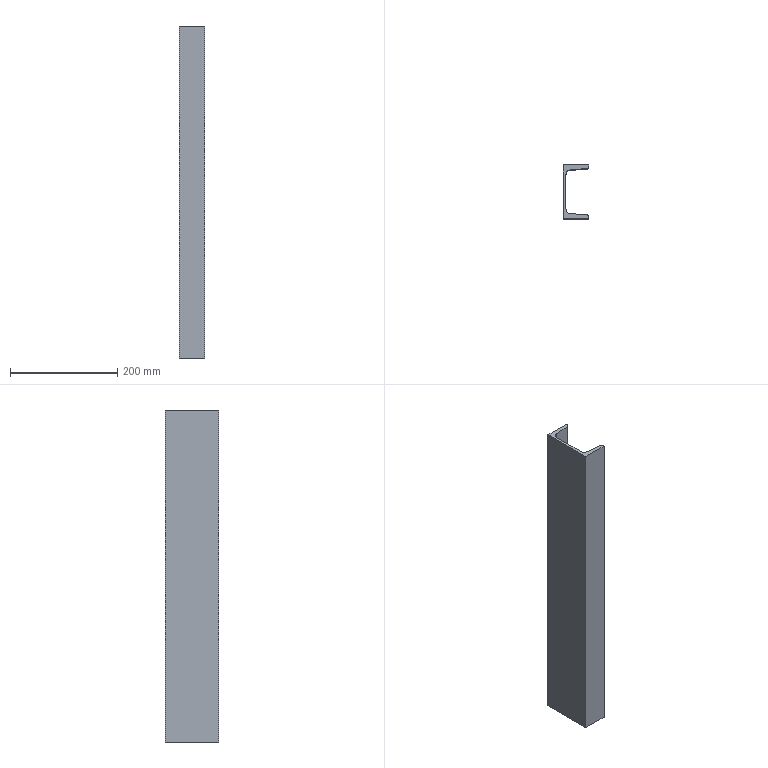Part | NX | features BREP 1 | 1 solid | 20 faces | box 48 x 100 x 620 mm | volume 770701 mm3 | cylinder 10 | plane 10 | commonest cylinder face diameters 14 x6 8.4 x2 17 x2
STEP:
#1=CARTESIAN_POINT('',(30.,92.079,-177.));
#2=VERTEX_POINT('',#1);
#3=CARTESIAN_POINT('',(30.,92.079,-163.));
#4=VERTEX_POINT('',#3);
#5=CARTESIAN_POINT('',(30.,92.079,-177.));
#6=CARTESIAN_POINT('',(16.,90.926,-177.));
#7=CARTESIAN_POINT('',(16.,90.926,-163.));
#8=CARTESIAN_POINT('',(30.,92.079,-163.));
#9=(BOUNDED_CURVE()B_SPLINE_CURVE(3,(#5,#6,#7,#8),.UNSPECIFIED.,.F.,.F.)B_SPLINE_CURVE_WITH_KNOTS((4,4),(0.,1.),.PIECEWISE_BEZIER_KNOTS.)CURVE()GEOMETRIC_REPRESENTATION_ITEM()RATIONAL_B_SPLINE_CURVE((1.,0.3333,0.3333,1.))REPRESENTATION_ITEM(''));
#10=EDGE_CURVE('',#2,#4,#9,.T.);
#11=ORIENTED_EDGE('',*,*,#10,.F.);
#12=CARTESIAN_POINT('',(30.,100.,-177.));
#13=VERTEX_POINT('',#12);
#14=CARTESIAN_POINT('',(30.,70.,-177.));
#15=DIRECTION('',(0.,1.,0.));
#16=VECTOR('',#15,1000.);
#17=LINE('',#14,#16);
#18=EDGE_CURVE('',#2,#13,#17,.T.);
#19=ORIENTED_EDGE('',*,*,#18,.T.);
#20=CARTESIAN_POINT('',(30.,100.,-163.));
#21=VERTEX_POINT('',#20);
#22=CARTESIAN_POINT('',(30.,100.,-170.));
#23=DIRECTION('',(0.,1.,0.));
#24=DIRECTION('',(0.,0.,1.));
#25=AXIS2_PLACEMENT_3D('',#22,#23,#24);
#26=CIRCLE('',#25,7.);
#27=EDGE_CURVE('',#13,#21,#26,.T.);
#28=ORIENTED_EDGE('',*,*,#27,.T.);
#29=CARTESIAN_POINT('',(30.,70.,-163.));
#30=DIRECTION('',(0.,1.,0.));
#31=VECTOR('',#30,1000.);
#32=LINE('',#29,#31);
#33=EDGE_CURVE('',#4,#21,#32,.T.);
#34=ORIENTED_EDGE('',*,*,#33,.F.);
#35=EDGE_LOOP('',(#11,#19,#28,#34));
#36=FACE_BOUND('',#35,.T.);
#37=CARTESIAN_POINT('',(30.,70.,-170.));
#38=DIRECTION('',(0.,1.,0.));
#39=DIRECTION('',(0.,0.,-1.));
#40=AXIS2_PLACEMENT_3D('',#37,#38,#39);
#41=CYLINDRICAL_SURFACE('',#40,7.);
#42=ADVANCED_FACE('',(#36),#41,.F.);
#43=CARTESIAN_POINT('',(30.,92.079,163.));
#44=VERTEX_POINT('',#43);
#45=CARTESIAN_POINT('',(30.,92.079,177.));
#46=VERTEX_POINT('',#45);
#47=CARTESIAN_POINT('',(30.,92.079,163.));
#48=CARTESIAN_POINT('',(16.,90.926,163.));
#49=CARTESIAN_POINT('',(16.,90.926,177.));
#50=CARTESIAN_POINT('',(30.,92.079,177.));
#51=(BOUNDED_CURVE()B_SPLINE_CURVE(3,(#47,#48,#49,#50),.UNSPECIFIED.,.F.,.F.)B_SPLINE_CURVE_WITH_KNOTS((4,4),(0.,1.),.PIECEWISE_BEZIER_KNOTS.)CURVE()GEOMETRIC_REPRESENTATION_ITEM()RATIONAL_B_SPLINE_CURVE((1.,0.3333,0.3333,1.))REPRESENTATION_ITEM(''));
#52=EDGE_CURVE('',#44,#46,#51,.T.);
#53=ORIENTED_EDGE('',*,*,#52,.F.);
#54=CARTESIAN_POINT('',(30.,100.,163.));
#55=VERTEX_POINT('',#54);
#56=CARTESIAN_POINT('',(30.,70.,163.));
#57=DIRECTION('',(0.,1.,0.));
#58=VECTOR('',#57,1000.);
#59=LINE('',#56,#58);
#60=EDGE_CURVE('',#44,#55,#59,.T.);
#61=ORIENTED_EDGE('',*,*,#60,.T.);
#62=CARTESIAN_POINT('',(30.,100.,177.));
#63=VERTEX_POINT('',#62);
#64=CARTESIAN_POINT('',(30.,100.,170.));
#65=DIRECTION('',(0.,1.,0.));
#66=DIRECTION('',(0.,0.,1.));
#67=AXIS2_PLACEMENT_3D('',#64,#65,#66);
#68=CIRCLE('',#67,7.);
#69=EDGE_CURVE('',#55,#63,#68,.T.);
#70=ORIENTED_EDGE('',*,*,#69,.T.);
#71=CARTESIAN_POINT('',(30.,70.,177.));
#72=DIRECTION('',(0.,1.,0.));
#73=VECTOR('',#72,1000.);
#74=LINE('',#71,#73);
#75=EDGE_CURVE('',#46,#63,#74,.T.);
#76=ORIENTED_EDGE('',*,*,#75,.F.);
#77=EDGE_LOOP('',(#53,#61,#70,#76));
#78=FACE_BOUND('',#77,.T.);
#79=CARTESIAN_POINT('',(30.,70.,170.));
#80=DIRECTION('',(0.,1.,0.));
#81=DIRECTION('',(0.,0.,-1.));
#82=AXIS2_PLACEMENT_3D('',#79,#80,#81);
#83=CYLINDRICAL_SURFACE('',#82,7.);
#84=ADVANCED_FACE('',(#78),#83,.F.);
#85=CARTESIAN_POINT('',(30.,92.079,-7.));
#86=VERTEX_POINT('',#85);
#87=CARTESIAN_POINT('',(30.,92.079,7.));
#88=VERTEX_POINT('',#87);
#89=CARTESIAN_POINT('',(30.,92.079,-7.));
#90=CARTESIAN_POINT('',(16.,90.926,-7.));
#91=CARTESIAN_POINT('',(16.,90.926,7.));
#92=CARTESIAN_POINT('',(30.,92.079,7.));
#93=(BOUNDED_CURVE()B_SPLINE_CURVE(3,(#89,#90,#91,#92),.UNSPECIFIED.,.F.,.F.)B_SPLINE_CURVE_WITH_KNOTS((4,4),(0.,1.),.PIECEWISE_BEZIER_KNOTS.)CURVE()GEOMETRIC_REPRESENTATION_ITEM()RATIONAL_B_SPLINE_CURVE((1.,0.3333,0.3333,1.))REPRESENTATION_ITEM(''));
#94=EDGE_CURVE('',#86,#88,#93,.T.);
#95=ORIENTED_EDGE('',*,*,#94,.F.);
#96=CARTESIAN_POINT('',(30.,100.,-7.));
#97=VERTEX_POINT('',#96);
#98=CARTESIAN_POINT('',(30.,70.,-7.));
#99=DIRECTION('',(0.,1.,0.));
#100=VECTOR('',#99,1000.);
#101=LINE('',#98,#100);
#102=EDGE_CURVE('',#86,#97,#101,.T.);
#103=ORIENTED_EDGE('',*,*,#102,.T.);
#104=CARTESIAN_POINT('',(30.,100.,7.));
#105=VERTEX_POINT('',#104);
#106=CARTESIAN_POINT('',(30.,100.,0.));
#107=DIRECTION('',(0.,1.,0.));
#108=DIRECTION('',(0.,0.,1.));
#109=AXIS2_PLACEMENT_3D('',#106,#107,#108);
#110=CIRCLE('',#109,7.);
#111=EDGE_CURVE('',#97,#105,#110,.T.);
#112=ORIENTED_EDGE('',*,*,#111,.T.);
#113=CARTESIAN_POINT('',(30.,70.,7.));
#114=DIRECTION('',(0.,1.,0.));
#115=VECTOR('',#114,1000.);
#116=LINE('',#113,#115);
#117=EDGE_CURVE('',#88,#105,#116,.T.);
#118=ORIENTED_EDGE('',*,*,#117,.F.);
#119=EDGE_LOOP('',(#95,#103,#112,#118));
#120=FACE_BOUND('',#119,.T.);
#121=CARTESIAN_POINT('',(30.,70.,0.));
#122=DIRECTION('',(0.,1.,0.));
#123=DIRECTION('',(0.,0.,-1.));
#124=AXIS2_PLACEMENT_3D('',#121,#122,#123);
#125=CYLINDRICAL_SURFACE('',#124,7.);
#126=ADVANCED_FACE('',(#120),#125,.F.);
#127=CARTESIAN_POINT('',(0.,0.,-310.));
#128=VERTEX_POINT('',#127);
#129=CARTESIAN_POINT('',(48.,0.,-310.));
#130=VERTEX_POINT('',#129);
#131=CARTESIAN_POINT('',(0.,0.,-310.));
#132=DIRECTION('',(1.,0.,0.));
#133=VECTOR('',#132,1000.);
#134=LINE('',#131,#133);
#135=EDGE_CURVE('',#128,#130,#134,.T.);
#136=ORIENTED_EDGE('',*,*,#135,.T.);
#137=CARTESIAN_POINT('',(48.,0.,310.));
#138=VERTEX_POINT('',#137);
#139=CARTESIAN_POINT('',(48.,0.,310.));
#140=DIRECTION('',(0.,0.,-1.));
#141=VECTOR('',#140,1000.);
#142=LINE('',#139,#141);
#143=EDGE_CURVE('',#138,#130,#142,.T.);
#144=ORIENTED_EDGE('',*,*,#143,.F.);
#145=CARTESIAN_POINT('',(0.,0.,310.));
#146=VERTEX_POINT('',#145);
#147=CARTESIAN_POINT('',(0.,0.,310.));
#148=DIRECTION('',(1.,0.,0.));
#149=VECTOR('',#148,1000.);
#150=LINE('',#147,#149);
#151=EDGE_CURVE('',#146,#138,#150,.T.);
#152=ORIENTED_EDGE('',*,*,#151,.F.);
#153=CARTESIAN_POINT('',(0.,0.,310.));
#154=DIRECTION('',(0.,0.,-1.));
#155=VECTOR('',#154,1000.);
#156=LINE('',#153,#155);
#157=EDGE_CURVE('',#146,#128,#156,.T.);
#158=ORIENTED_EDGE('',*,*,#157,.T.);
#159=EDGE_LOOP('',(#136,#144,#152,#158));
#160=FACE_BOUND('',#159,.T.);
#161=CARTESIAN_POINT('',(0.,0.,310.));
#162=DIRECTION('',(0.,1.,0.));
#163=DIRECTION('',(0.,0.,-1.));
#164=AXIS2_PLACEMENT_3D('',#161,#162,#163);
#165=PLANE('',#164);
#166=ADVANCED_FACE('',(#160),#165,.F.);
#167=CARTESIAN_POINT('',(48.,2.585,-310.));
#168=VERTEX_POINT('',#167);
#169=CARTESIAN_POINT('',(48.,0.,-310.));
#170=DIRECTION('',(0.,1.,0.));
#171=VECTOR('',#170,1000.);
#172=LINE('',#169,#171);
#173=EDGE_CURVE('',#130,#168,#172,.T.);
#174=ORIENTED_EDGE('',*,*,#173,.T.);
#175=CARTESIAN_POINT('',(48.,2.585,310.));
#176=VERTEX_POINT('',#175);
#177=CARTESIAN_POINT('',(48.,2.585,310.));
#178=DIRECTION('',(0.,0.,-1.));
#179=VECTOR('',#178,1000.);
#180=LINE('',#177,#179);
#181=EDGE_CURVE('',#176,#168,#180,.T.);
#182=ORIENTED_EDGE('',*,*,#181,.F.);
#183=CARTESIAN_POINT('',(48.,0.,310.));
#184=DIRECTION('',(0.,1.,0.));
#185=VECTOR('',#184,1000.);
#186=LINE('',#183,#185);
#187=EDGE_CURVE('',#138,#176,#186,.T.);
#188=ORIENTED_EDGE('',*,*,#187,.F.);
#189=ORIENTED_EDGE('',*,*,#143,.T.);
#190=EDGE_LOOP('',(#174,#182,#188,#189));
#191=FACE_BOUND('',#190,.T.);
#192=CARTESIAN_POINT('',(48.,0.,310.));
#193=DIRECTION('',(-1.,0.,0.));
#194=DIRECTION('',(0.,0.,-1.));
#195=AXIS2_PLACEMENT_3D('',#192,#193,#194);
#196=PLANE('',#195);
#197=ADVANCED_FACE('',(#191),#196,.F.);
#198=CARTESIAN_POINT('',(43.8,6.785,-310.));
#199=VERTEX_POINT('',#198);
#200=CARTESIAN_POINT('',(43.8,2.585,-310.));
#201=DIRECTION('',(0.,0.,1.));
#202=DIRECTION('',(1.,0.,0.));
#203=AXIS2_PLACEMENT_3D('',#200,#201,#202);
#204=CIRCLE('',#203,4.2);
#205=EDGE_CURVE('',#168,#199,#204,.T.);
#206=ORIENTED_EDGE('',*,*,#205,.T.);
#207=CARTESIAN_POINT('',(43.8,6.785,310.));
#208=VERTEX_POINT('',#207);
#209=CARTESIAN_POINT('',(43.8,6.785,310.));
#210=DIRECTION('',(0.,0.,-1.));
#211=VECTOR('',#210,1000.);
#212=LINE('',#209,#211);
#213=EDGE_CURVE('',#208,#199,#212,.T.);
#214=ORIENTED_EDGE('',*,*,#213,.F.);
#215=CARTESIAN_POINT('',(43.8,2.585,310.));
#216=DIRECTION('',(0.,0.,1.));
#217=DIRECTION('',(1.,0.,0.));
#218=AXIS2_PLACEMENT_3D('',#215,#216,#217);
#219=CIRCLE('',#218,4.2);
#220=EDGE_CURVE('',#176,#208,#219,.T.);
#221=ORIENTED_EDGE('',*,*,#220,.F.);
#222=ORIENTED_EDGE('',*,*,#181,.T.);
#223=EDGE_LOOP('',(#206,#214,#221,#222));
#224=FACE_BOUND('',#223,.T.);
#225=CARTESIAN_POINT('',(43.8,2.585,310.));
#226=DIRECTION('',(0.,0.,-1.));
#227=DIRECTION('',(1.,0.,0.));
#228=AXIS2_PLACEMENT_3D('',#225,#226,#227);
#229=CYLINDRICAL_SURFACE('',#228,4.2);
#230=ADVANCED_FACE('',(#224),#229,.T.);
#231=CARTESIAN_POINT('',(13.8,9.255,-310.));
#232=VERTEX_POINT('',#231);
#233=CARTESIAN_POINT('',(43.8,6.785,-310.));
#234=DIRECTION('',(-0.9966,0.08206,0.));
#235=VECTOR('',#234,1000.);
#236=LINE('',#233,#235);
#237=EDGE_CURVE('',#199,#232,#236,.T.);
#238=ORIENTED_EDGE('',*,*,#237,.T.);
#239=CARTESIAN_POINT('',(13.8,9.255,310.));
#240=VERTEX_POINT('',#239);
#241=CARTESIAN_POINT('',(13.8,9.255,310.));
#242=DIRECTION('',(0.,0.,-1.));
#243=VECTOR('',#242,1000.);
#244=LINE('',#241,#243);
#245=EDGE_CURVE('',#240,#232,#244,.T.);
#246=ORIENTED_EDGE('',*,*,#245,.F.);
#247=CARTESIAN_POINT('',(43.8,6.785,310.));
#248=DIRECTION('',(-0.9966,0.08206,0.));
#249=VECTOR('',#248,1000.);
#250=LINE('',#247,#249);
#251=EDGE_CURVE('',#208,#240,#250,.T.);
#252=ORIENTED_EDGE('',*,*,#251,.F.);
#253=ORIENTED_EDGE('',*,*,#213,.T.);
#254=EDGE_LOOP('',(#238,#246,#252,#253));
#255=FACE_BOUND('',#254,.T.);
#256=CARTESIAN_POINT('',(43.8,6.785,310.));
#257=DIRECTION('',(-0.08206,-0.9966,0.));
#258=DIRECTION('',(-0.9966,0.08206,0.));
#259=AXIS2_PLACEMENT_3D('',#256,#257,#258);
#260=PLANE('',#259);
#261=ADVANCED_FACE('',(#255),#260,.F.);
#262=CARTESIAN_POINT('',(5.3,17.755,-310.));
#263=VERTEX_POINT('',#262);
#264=CARTESIAN_POINT('',(13.8,17.755,-310.));
#265=DIRECTION('',(0.,0.,-1.));
#266=DIRECTION('',(1.,0.,0.));
#267=AXIS2_PLACEMENT_3D('',#264,#265,#266);
#268=CIRCLE('',#267,8.5);
#269=EDGE_CURVE('',#232,#263,#268,.T.);
#270=ORIENTED_EDGE('',*,*,#269,.T.);
#271=CARTESIAN_POINT('',(5.3,17.755,310.));
#272=VERTEX_POINT('',#271);
#273=CARTESIAN_POINT('',(5.3,17.755,310.));
#274=DIRECTION('',(0.,0.,-1.));
#275=VECTOR('',#274,1000.);
#276=LINE('',#273,#275);
#277=EDGE_CURVE('',#272,#263,#276,.T.);
#278=ORIENTED_EDGE('',*,*,#277,.F.);
#279=CARTESIAN_POINT('',(13.8,17.755,310.));
#280=DIRECTION('',(0.,0.,-1.));
#281=DIRECTION('',(1.,0.,0.));
#282=AXIS2_PLACEMENT_3D('',#279,#280,#281);
#283=CIRCLE('',#282,8.5);
#284=EDGE_CURVE('',#240,#272,#283,.T.);
#285=ORIENTED_EDGE('',*,*,#284,.F.);
#286=ORIENTED_EDGE('',*,*,#245,.T.);
#287=EDGE_LOOP('',(#270,#278,#285,#286));
#288=FACE_BOUND('',#287,.T.);
#289=CARTESIAN_POINT('',(13.8,17.755,310.));
#290=DIRECTION('',(0.,0.,-1.));
#291=DIRECTION('',(1.,0.,0.));
#292=AXIS2_PLACEMENT_3D('',#289,#290,#291);
#293=CYLINDRICAL_SURFACE('',#292,8.5);
#294=ADVANCED_FACE('',(#288),#293,.F.);
#295=CARTESIAN_POINT('',(5.3,82.245,-310.));
#296=VERTEX_POINT('',#295);
#297=CARTESIAN_POINT('',(5.3,17.755,-310.));
#298=DIRECTION('',(0.,1.,0.));
#299=VECTOR('',#298,1000.);
#300=LINE('',#297,#299);
#301=EDGE_CURVE('',#263,#296,#300,.T.);
#302=ORIENTED_EDGE('',*,*,#301,.T.);
#303=CARTESIAN_POINT('',(5.3,82.245,310.));
#304=VERTEX_POINT('',#303);
#305=CARTESIAN_POINT('',(5.3,82.245,310.));
#306=DIRECTION('',(0.,0.,-1.));
#307=VECTOR('',#306,1000.);
#308=LINE('',#305,#307);
#309=EDGE_CURVE('',#304,#296,#308,.T.);
#310=ORIENTED_EDGE('',*,*,#309,.F.);
#311=CARTESIAN_POINT('',(5.3,17.755,310.));
#312=DIRECTION('',(0.,1.,0.));
#313=VECTOR('',#312,1000.);
#314=LINE('',#311,#313);
#315=EDGE_CURVE('',#272,#304,#314,.T.);
#316=ORIENTED_EDGE('',*,*,#315,.F.);
#317=ORIENTED_EDGE('',*,*,#277,.T.);
#318=EDGE_LOOP('',(#302,#310,#316,#317));
#319=FACE_BOUND('',#318,.T.);
#320=CARTESIAN_POINT('',(5.3,17.755,310.));
#321=DIRECTION('',(-1.,0.,0.));
#322=DIRECTION('',(0.,0.,-1.));
#323=AXIS2_PLACEMENT_3D('',#320,#321,#322);
#324=PLANE('',#323);
#325=ADVANCED_FACE('',(#319),#324,.F.);
#326=CARTESIAN_POINT('',(13.8,90.745,-310.));
#327=VERTEX_POINT('',#326);
#328=CARTESIAN_POINT('',(13.8,82.245,-310.));
#329=DIRECTION('',(0.,0.,-1.));
#330=DIRECTION('',(-1.,0.,0.));
#331=AXIS2_PLACEMENT_3D('',#328,#329,#330);
#332=CIRCLE('',#331,8.5);
#333=EDGE_CURVE('',#296,#327,#332,.T.);
#334=ORIENTED_EDGE('',*,*,#333,.T.);
#335=CARTESIAN_POINT('',(13.8,90.745,310.));
#336=VERTEX_POINT('',#335);
#337=CARTESIAN_POINT('',(13.8,90.745,310.));
#338=DIRECTION('',(0.,0.,-1.));
#339=VECTOR('',#338,1000.);
#340=LINE('',#337,#339);
#341=EDGE_CURVE('',#336,#327,#340,.T.);
#342=ORIENTED_EDGE('',*,*,#341,.F.);
#343=CARTESIAN_POINT('',(13.8,82.245,310.));
#344=DIRECTION('',(0.,0.,-1.));
#345=DIRECTION('',(-1.,0.,0.));
#346=AXIS2_PLACEMENT_3D('',#343,#344,#345);
#347=CIRCLE('',#346,8.5);
#348=EDGE_CURVE('',#304,#336,#347,.T.);
#349=ORIENTED_EDGE('',*,*,#348,.F.);
#350=ORIENTED_EDGE('',*,*,#309,.T.);
#351=EDGE_LOOP('',(#334,#342,#349,#350));
#352=FACE_BOUND('',#351,.T.);
#353=CARTESIAN_POINT('',(13.8,82.245,310.));
#354=DIRECTION('',(0.,0.,-1.));
#355=DIRECTION('',(1.,0.,0.));
#356=AXIS2_PLACEMENT_3D('',#353,#354,#355);
#357=CYLINDRICAL_SURFACE('',#356,8.5);
#358=ADVANCED_FACE('',(#352),#357,.F.);
#359=CARTESIAN_POINT('',(30.,92.079,-163.));
#360=CARTESIAN_POINT('',(44.,93.231,-163.));
#361=CARTESIAN_POINT('',(44.,93.231,-177.));
#362=CARTESIAN_POINT('',(30.,92.079,-177.));
#363=(BOUNDED_CURVE()B_SPLINE_CURVE(3,(#359,#360,#361,#362),.UNSPECIFIED.,.F.,.F.)B_SPLINE_CURVE_WITH_KNOTS((4,4),(0.,1.),.PIECEWISE_BEZIER_KNOTS.)CURVE()GEOMETRIC_REPRESENTATION_ITEM()RATIONAL_B_SPLINE_CURVE((1.,0.3333,0.3333,1.))REPRESENTATION_ITEM(''));
#364=EDGE_CURVE('',#4,#2,#363,.T.);
#365=ORIENTED_EDGE('',*,*,#364,.T.);
#366=ORIENTED_EDGE('',*,*,#10,.T.);
#367=EDGE_LOOP('',(#365,#366));
#368=FACE_BOUND('',#367,.T.);
#369=CARTESIAN_POINT('',(30.,92.079,177.));
#370=CARTESIAN_POINT('',(44.,93.231,177.));
#371=CARTESIAN_POINT('',(44.,93.231,163.));
#372=CARTESIAN_POINT('',(30.,92.079,163.));
#373=(BOUNDED_CURVE()B_SPLINE_CURVE(3,(#369,#370,#371,#372),.UNSPECIFIED.,.F.,.F.)B_SPLINE_CURVE_WITH_KNOTS((4,4),(0.,1.),.PIECEWISE_BEZIER_KNOTS.)CURVE()GEOMETRIC_REPRESENTATION_ITEM()RATIONAL_B_SPLINE_CURVE((1.,0.3333,0.3333,1.))REPRESENTATION_ITEM(''));
#374=EDGE_CURVE('',#46,#44,#373,.T.);
#375=ORIENTED_EDGE('',*,*,#374,.T.);
#376=ORIENTED_EDGE('',*,*,#52,.T.);
#377=EDGE_LOOP('',(#375,#376));
#378=FACE_BOUND('',#377,.T.);
#379=CARTESIAN_POINT('',(30.,92.079,7.));
#380=CARTESIAN_POINT('',(44.,93.231,7.));
#381=CARTESIAN_POINT('',(44.,93.231,-7.));
#382=CARTESIAN_POINT('',(30.,92.079,-7.));
#383=(BOUNDED_CURVE()B_SPLINE_CURVE(3,(#379,#380,#381,#382),.UNSPECIFIED.,.F.,.F.)B_SPLINE_CURVE_WITH_KNOTS((4,4),(0.,1.),.PIECEWISE_BEZIER_KNOTS.)CURVE()GEOMETRIC_REPRESENTATION_ITEM()RATIONAL_B_SPLINE_CURVE((1.,0.3333,0.3333,1.))REPRESENTATION_ITEM(''));
#384=EDGE_CURVE('',#88,#86,#383,.T.);
#385=ORIENTED_EDGE('',*,*,#384,.T.);
#386=ORIENTED_EDGE('',*,*,#94,.T.);
#387=EDGE_LOOP('',(#385,#386));
#388=FACE_BOUND('',#387,.T.);
#389=CARTESIAN_POINT('',(43.8,93.215,-310.));
#390=VERTEX_POINT('',#389);
#391=CARTESIAN_POINT('',(43.8,93.215,-310.));
#392=DIRECTION('',(0.9966,0.08206,0.));
#393=VECTOR('',#392,1000.);
#394=LINE('',#391,#393);
#395=EDGE_CURVE('',#327,#390,#394,.T.);
#396=ORIENTED_EDGE('',*,*,#395,.T.);
#397=CARTESIAN_POINT('',(43.8,93.215,310.));
#398=VERTEX_POINT('',#397);
#399=CARTESIAN_POINT('',(43.8,93.215,310.));
#400=DIRECTION('',(0.,0.,-1.));
#401=VECTOR('',#400,1000.);
#402=LINE('',#399,#401);
#403=EDGE_CURVE('',#398,#390,#402,.T.);
#404=ORIENTED_EDGE('',*,*,#403,.F.);
#405=CARTESIAN_POINT('',(43.8,93.215,310.));
#406=DIRECTION('',(0.9966,0.08206,0.));
#407=VECTOR('',#406,1000.);
#408=LINE('',#405,#407);
#409=EDGE_CURVE('',#336,#398,#408,.T.);
#410=ORIENTED_EDGE('',*,*,#409,.F.);
#411=ORIENTED_EDGE('',*,*,#341,.T.);
#412=EDGE_LOOP('',(#396,#404,#410,#411));
#413=FACE_BOUND('',#412,.T.);
#414=CARTESIAN_POINT('',(43.8,93.215,310.));
#415=DIRECTION('',(-0.08206,0.9966,0.));
#416=DIRECTION('',(0.9966,0.08206,0.));
#417=AXIS2_PLACEMENT_3D('',#414,#415,#416);
#418=PLANE('',#417);
#419=ADVANCED_FACE('',(#368,#378,#388,#413),#418,.F.);
#420=CARTESIAN_POINT('',(48.,97.415,-310.));
#421=VERTEX_POINT('',#420);
#422=CARTESIAN_POINT('',(43.8,97.415,-310.));
#423=DIRECTION('',(0.,0.,1.));
#424=DIRECTION('',(-1.,0.,0.));
#425=AXIS2_PLACEMENT_3D('',#422,#423,#424);
#426=CIRCLE('',#425,4.2);
#427=EDGE_CURVE('',#390,#421,#426,.T.);
#428=ORIENTED_EDGE('',*,*,#427,.T.);
#429=CARTESIAN_POINT('',(48.,97.415,310.));
#430=VERTEX_POINT('',#429);
#431=CARTESIAN_POINT('',(48.,97.415,310.));
#432=DIRECTION('',(0.,0.,-1.));
#433=VECTOR('',#432,1000.);
#434=LINE('',#431,#433);
#435=EDGE_CURVE('',#430,#421,#434,.T.);
#436=ORIENTED_EDGE('',*,*,#435,.F.);
#437=CARTESIAN_POINT('',(43.8,97.415,310.));
#438=DIRECTION('',(0.,0.,1.));
#439=DIRECTION('',(-1.,0.,0.));
#440=AXIS2_PLACEMENT_3D('',#437,#438,#439);
#441=CIRCLE('',#440,4.2);
#442=EDGE_CURVE('',#398,#430,#441,.T.);
#443=ORIENTED_EDGE('',*,*,#442,.F.);
#444=ORIENTED_EDGE('',*,*,#403,.T.);
#445=EDGE_LOOP('',(#428,#436,#443,#444));
#446=FACE_BOUND('',#445,.T.);
#447=CARTESIAN_POINT('',(43.8,97.415,310.));
#448=DIRECTION('',(0.,0.,-1.));
#449=DIRECTION('',(1.,0.,0.));
#450=AXIS2_PLACEMENT_3D('',#447,#448,#449);
#451=CYLINDRICAL_SURFACE('',#450,4.2);
#452=ADVANCED_FACE('',(#446),#451,.T.);
#453=CARTESIAN_POINT('',(48.,100.,-310.));
#454=VERTEX_POINT('',#453);
#455=CARTESIAN_POINT('',(48.,100.,-310.));
#456=DIRECTION('',(0.,1.,0.));
#457=VECTOR('',#456,1000.);
#458=LINE('',#455,#457);
#459=EDGE_CURVE('',#421,#454,#458,.T.);
#460=ORIENTED_EDGE('',*,*,#459,.T.);
#461=CARTESIAN_POINT('',(48.,100.,310.));
#462=VERTEX_POINT('',#461);
#463=CARTESIAN_POINT('',(48.,100.,310.));
#464=DIRECTION('',(0.,0.,-1.));
#465=VECTOR('',#464,1000.);
#466=LINE('',#463,#465);
#467=EDGE_CURVE('',#462,#454,#466,.T.);
#468=ORIENTED_EDGE('',*,*,#467,.F.);
#469=CARTESIAN_POINT('',(48.,100.,310.));
#470=DIRECTION('',(0.,1.,0.));
#471=VECTOR('',#470,1000.);
#472=LINE('',#469,#471);
#473=EDGE_CURVE('',#430,#462,#472,.T.);
#474=ORIENTED_EDGE('',*,*,#473,.F.);
#475=ORIENTED_EDGE('',*,*,#435,.T.);
#476=EDGE_LOOP('',(#460,#468,#474,#475));
#477=FACE_BOUND('',#476,.T.);
#478=CARTESIAN_POINT('',(48.,100.,310.));
#479=DIRECTION('',(-1.,0.,0.));
#480=DIRECTION('',(0.,0.,-1.));
#481=AXIS2_PLACEMENT_3D('',#478,#479,#480);
#482=PLANE('',#481);
#483=ADVANCED_FACE('',(#477),#482,.F.);
#484=CARTESIAN_POINT('',(30.,100.,-170.));
#485=DIRECTION('',(0.,1.,0.));
#486=DIRECTION('',(0.,0.,1.));
#487=AXIS2_PLACEMENT_3D('',#484,#485,#486);
#488=CIRCLE('',#487,7.);
#489=EDGE_CURVE('',#21,#13,#488,.T.);
#490=ORIENTED_EDGE('',*,*,#489,.F.);
#491=ORIENTED_EDGE('',*,*,#27,.F.);
#492=EDGE_LOOP('',(#490,#491));
#493=FACE_BOUND('',#492,.T.);
#494=CARTESIAN_POINT('',(30.,100.,170.));
#495=DIRECTION('',(0.,1.,0.));
#496=DIRECTION('',(0.,0.,1.));
#497=AXIS2_PLACEMENT_3D('',#494,#495,#496);
#498=CIRCLE('',#497,7.);
#499=EDGE_CURVE('',#63,#55,#498,.T.);
#500=ORIENTED_EDGE('',*,*,#499,.F.);
#501=ORIENTED_EDGE('',*,*,#69,.F.);
#502=EDGE_LOOP('',(#500,#501));
#503=FACE_BOUND('',#502,.T.);
#504=CARTESIAN_POINT('',(30.,100.,0.));
#505=DIRECTION('',(0.,1.,0.));
#506=DIRECTION('',(0.,0.,1.));
#507=AXIS2_PLACEMENT_3D('',#504,#505,#506);
#508=CIRCLE('',#507,7.);
#509=EDGE_CURVE('',#105,#97,#508,.T.);
#510=ORIENTED_EDGE('',*,*,#509,.F.);
#511=ORIENTED_EDGE('',*,*,#111,.F.);
#512=EDGE_LOOP('',(#510,#511));
#513=FACE_BOUND('',#512,.T.);
#514=CARTESIAN_POINT('',(0.,100.,-310.));
#515=VERTEX_POINT('',#514);
#516=CARTESIAN_POINT('',(0.,100.,-310.));
#517=DIRECTION('',(-1.,0.,0.));
#518=VECTOR('',#517,1000.);
#519=LINE('',#516,#518);
#520=EDGE_CURVE('',#454,#515,#519,.T.);
#521=ORIENTED_EDGE('',*,*,#520,.T.);
#522=CARTESIAN_POINT('',(0.,100.,310.));
#523=VERTEX_POINT('',#522);
#524=CARTESIAN_POINT('',(0.,100.,310.));
#525=DIRECTION('',(0.,0.,-1.));
#526=VECTOR('',#525,1000.);
#527=LINE('',#524,#526);
#528=EDGE_CURVE('',#523,#515,#527,.T.);
#529=ORIENTED_EDGE('',*,*,#528,.F.);
#530=CARTESIAN_POINT('',(0.,100.,310.));
#531=DIRECTION('',(-1.,0.,0.));
#532=VECTOR('',#531,1000.);
#533=LINE('',#530,#532);
#534=EDGE_CURVE('',#462,#523,#533,.T.);
#535=ORIENTED_EDGE('',*,*,#534,.F.);
#536=ORIENTED_EDGE('',*,*,#467,.T.);
#537=EDGE_LOOP('',(#521,#529,#535,#536));
#538=FACE_BOUND('',#537,.T.);
#539=CARTESIAN_POINT('',(0.,100.,310.));
#540=DIRECTION('',(0.,-1.,0.));
#541=DIRECTION('',(0.,0.,1.));
#542=AXIS2_PLACEMENT_3D('',#539,#540,#541);
#543=PLANE('',#542);
#544=ADVANCED_FACE('',(#493,#503,#513,#538),#543,.F.);
#545=CARTESIAN_POINT('',(0.,100.,-310.));
#546=DIRECTION('',(0.,-1.,0.));
#547=VECTOR('',#546,1000.);
#548=LINE('',#545,#547);
#549=EDGE_CURVE('',#515,#128,#548,.T.);
#550=ORIENTED_EDGE('',*,*,#549,.T.);
#551=ORIENTED_EDGE('',*,*,#157,.F.);
#552=CARTESIAN_POINT('',(0.,100.,310.));
#553=DIRECTION('',(0.,-1.,0.));
#554=VECTOR('',#553,1000.);
#555=LINE('',#552,#554);
#556=EDGE_CURVE('',#523,#146,#555,.T.);
#557=ORIENTED_EDGE('',*,*,#556,.F.);
#558=ORIENTED_EDGE('',*,*,#528,.T.);
#559=EDGE_LOOP('',(#550,#551,#557,#558));
#560=FACE_BOUND('',#559,.T.);
#561=CARTESIAN_POINT('',(0.,100.,310.));
#562=DIRECTION('',(1.,0.,0.));
#563=DIRECTION('',(0.,0.,1.));
#564=AXIS2_PLACEMENT_3D('',#561,#562,#563);
#565=PLANE('',#564);
#566=ADVANCED_FACE('',(#560),#565,.F.);
#567=ORIENTED_EDGE('',*,*,#151,.T.);
#568=ORIENTED_EDGE('',*,*,#187,.T.);
#569=ORIENTED_EDGE('',*,*,#220,.T.);
#570=ORIENTED_EDGE('',*,*,#251,.T.);
#571=ORIENTED_EDGE('',*,*,#284,.T.);
#572=ORIENTED_EDGE('',*,*,#315,.T.);
#573=ORIENTED_EDGE('',*,*,#348,.T.);
#574=ORIENTED_EDGE('',*,*,#409,.T.);
#575=ORIENTED_EDGE('',*,*,#442,.T.);
#576=ORIENTED_EDGE('',*,*,#473,.T.);
#577=ORIENTED_EDGE('',*,*,#534,.T.);
#578=ORIENTED_EDGE('',*,*,#556,.T.);
#579=EDGE_LOOP('',(#567,#568,#569,#570,#571,#572,#573,#574,#575,#576,#577,#578));
#580=FACE_BOUND('',#579,.T.);
#581=CARTESIAN_POINT('',(43.8,2.585,310.));
#582=DIRECTION('',(0.,0.,1.));
#583=DIRECTION('',(-1.,0.,0.));
#584=AXIS2_PLACEMENT_3D('',#581,#582,#583);
#585=PLANE('',#584);
#586=ADVANCED_FACE('',(#580),#585,.T.);
#587=ORIENTED_EDGE('',*,*,#135,.F.);
#588=ORIENTED_EDGE('',*,*,#549,.F.);
#589=ORIENTED_EDGE('',*,*,#520,.F.);
#590=ORIENTED_EDGE('',*,*,#459,.F.);
#591=ORIENTED_EDGE('',*,*,#427,.F.);
#592=ORIENTED_EDGE('',*,*,#395,.F.);
#593=ORIENTED_EDGE('',*,*,#333,.F.);
#594=ORIENTED_EDGE('',*,*,#301,.F.);
#595=ORIENTED_EDGE('',*,*,#269,.F.);
#596=ORIENTED_EDGE('',*,*,#237,.F.);
#597=ORIENTED_EDGE('',*,*,#205,.F.);
#598=ORIENTED_EDGE('',*,*,#173,.F.);
#599=EDGE_LOOP('',(#587,#588,#589,#590,#591,#592,#593,#594,#595,#596,#597,#598));
#600=FACE_BOUND('',#599,.T.);
#601=CARTESIAN_POINT('',(43.8,2.585,-310.));
#602=DIRECTION('',(0.,0.,1.));
#603=DIRECTION('',(-1.,0.,0.));
#604=AXIS2_PLACEMENT_3D('',#601,#602,#603);
#605=PLANE('',#604);
#606=ADVANCED_FACE('',(#600),#605,.F.);
#607=ORIENTED_EDGE('',*,*,#102,.F.);
#608=ORIENTED_EDGE('',*,*,#384,.F.);
#609=ORIENTED_EDGE('',*,*,#117,.T.);
#610=ORIENTED_EDGE('',*,*,#509,.T.);
#611=EDGE_LOOP('',(#607,#608,#609,#610));
#612=FACE_BOUND('',#611,.T.);
#613=CARTESIAN_POINT('',(30.,70.,0.));
#614=DIRECTION('',(0.,1.,0.));
#615=DIRECTION('',(0.,0.,-1.));
#616=AXIS2_PLACEMENT_3D('',#613,#614,#615);
#617=CYLINDRICAL_SURFACE('',#616,7.);
#618=ADVANCED_FACE('',(#612),#617,.F.);
#619=ORIENTED_EDGE('',*,*,#60,.F.);
#620=ORIENTED_EDGE('',*,*,#374,.F.);
#621=ORIENTED_EDGE('',*,*,#75,.T.);
#622=ORIENTED_EDGE('',*,*,#499,.T.);
#623=EDGE_LOOP('',(#619,#620,#621,#622));
#624=FACE_BOUND('',#623,.T.);
#625=CARTESIAN_POINT('',(30.,70.,170.));
#626=DIRECTION('',(0.,1.,0.));
#627=DIRECTION('',(0.,0.,-1.));
#628=AXIS2_PLACEMENT_3D('',#625,#626,#627);
#629=CYLINDRICAL_SURFACE('',#628,7.);
#630=ADVANCED_FACE('',(#624),#629,.F.);
#631=ORIENTED_EDGE('',*,*,#18,.F.);
#632=ORIENTED_EDGE('',*,*,#364,.F.);
#633=ORIENTED_EDGE('',*,*,#33,.T.);
#634=ORIENTED_EDGE('',*,*,#489,.T.);
#635=EDGE_LOOP('',(#631,#632,#633,#634));
#636=FACE_BOUND('',#635,.T.);
#637=CARTESIAN_POINT('',(30.,70.,-170.));
#638=DIRECTION('',(0.,1.,0.));
#639=DIRECTION('',(0.,0.,-1.));
#640=AXIS2_PLACEMENT_3D('',#637,#638,#639);
#641=CYLINDRICAL_SURFACE('',#640,7.);
#642=ADVANCED_FACE('',(#636),#641,.F.);
#643=CLOSED_SHELL('',(#42,#84,#126,#166,#197,#230,#261,#294,#325,#358,#419,#452,#483,#544,#566,#586,#606,#618,#630,#642));
#644=MANIFOLD_SOLID_BREP('',#643);
#645=(LENGTH_UNIT()NAMED_UNIT(*)SI_UNIT(.MILLI.,.METRE.));
#646=UNCERTAINTY_MEASURE_WITH_UNIT(LENGTH_MEASURE(0.00001),#645,'','');
#647=(NAMED_UNIT(*)PLANE_ANGLE_UNIT()SI_UNIT($,.RADIAN.));
#648=(NAMED_UNIT(*)SI_UNIT($,.STERADIAN.)SOLID_ANGLE_UNIT());
#649=(GEOMETRIC_REPRESENTATION_CONTEXT(3)GLOBAL_UNCERTAINTY_ASSIGNED_CONTEXT((#646))GLOBAL_UNIT_ASSIGNED_CONTEXT((#645,#647,#648))REPRESENTATION_CONTEXT('',''));
#650=ADVANCED_BREP_SHAPE_REPRESENTATION('',(#644),#649);